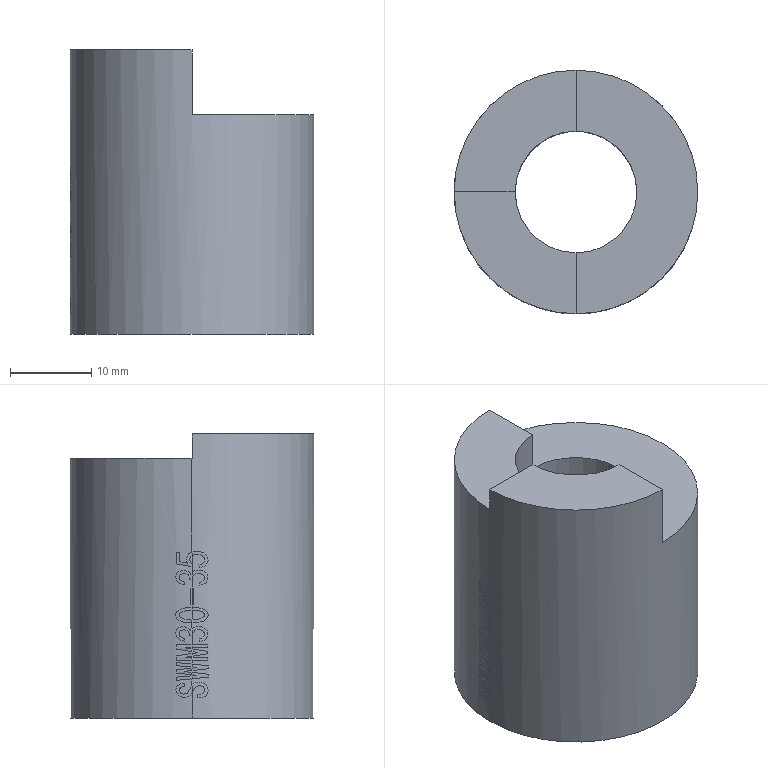Part | SolidWorks | features BaseBody 1 | 1 solid | 43 faces | box 30 x 30 x 35 mm | volume 16035 mm3 | cylinder 36 | plane 7 | commonest cylinder face diameters 30 x34 15.003 x2